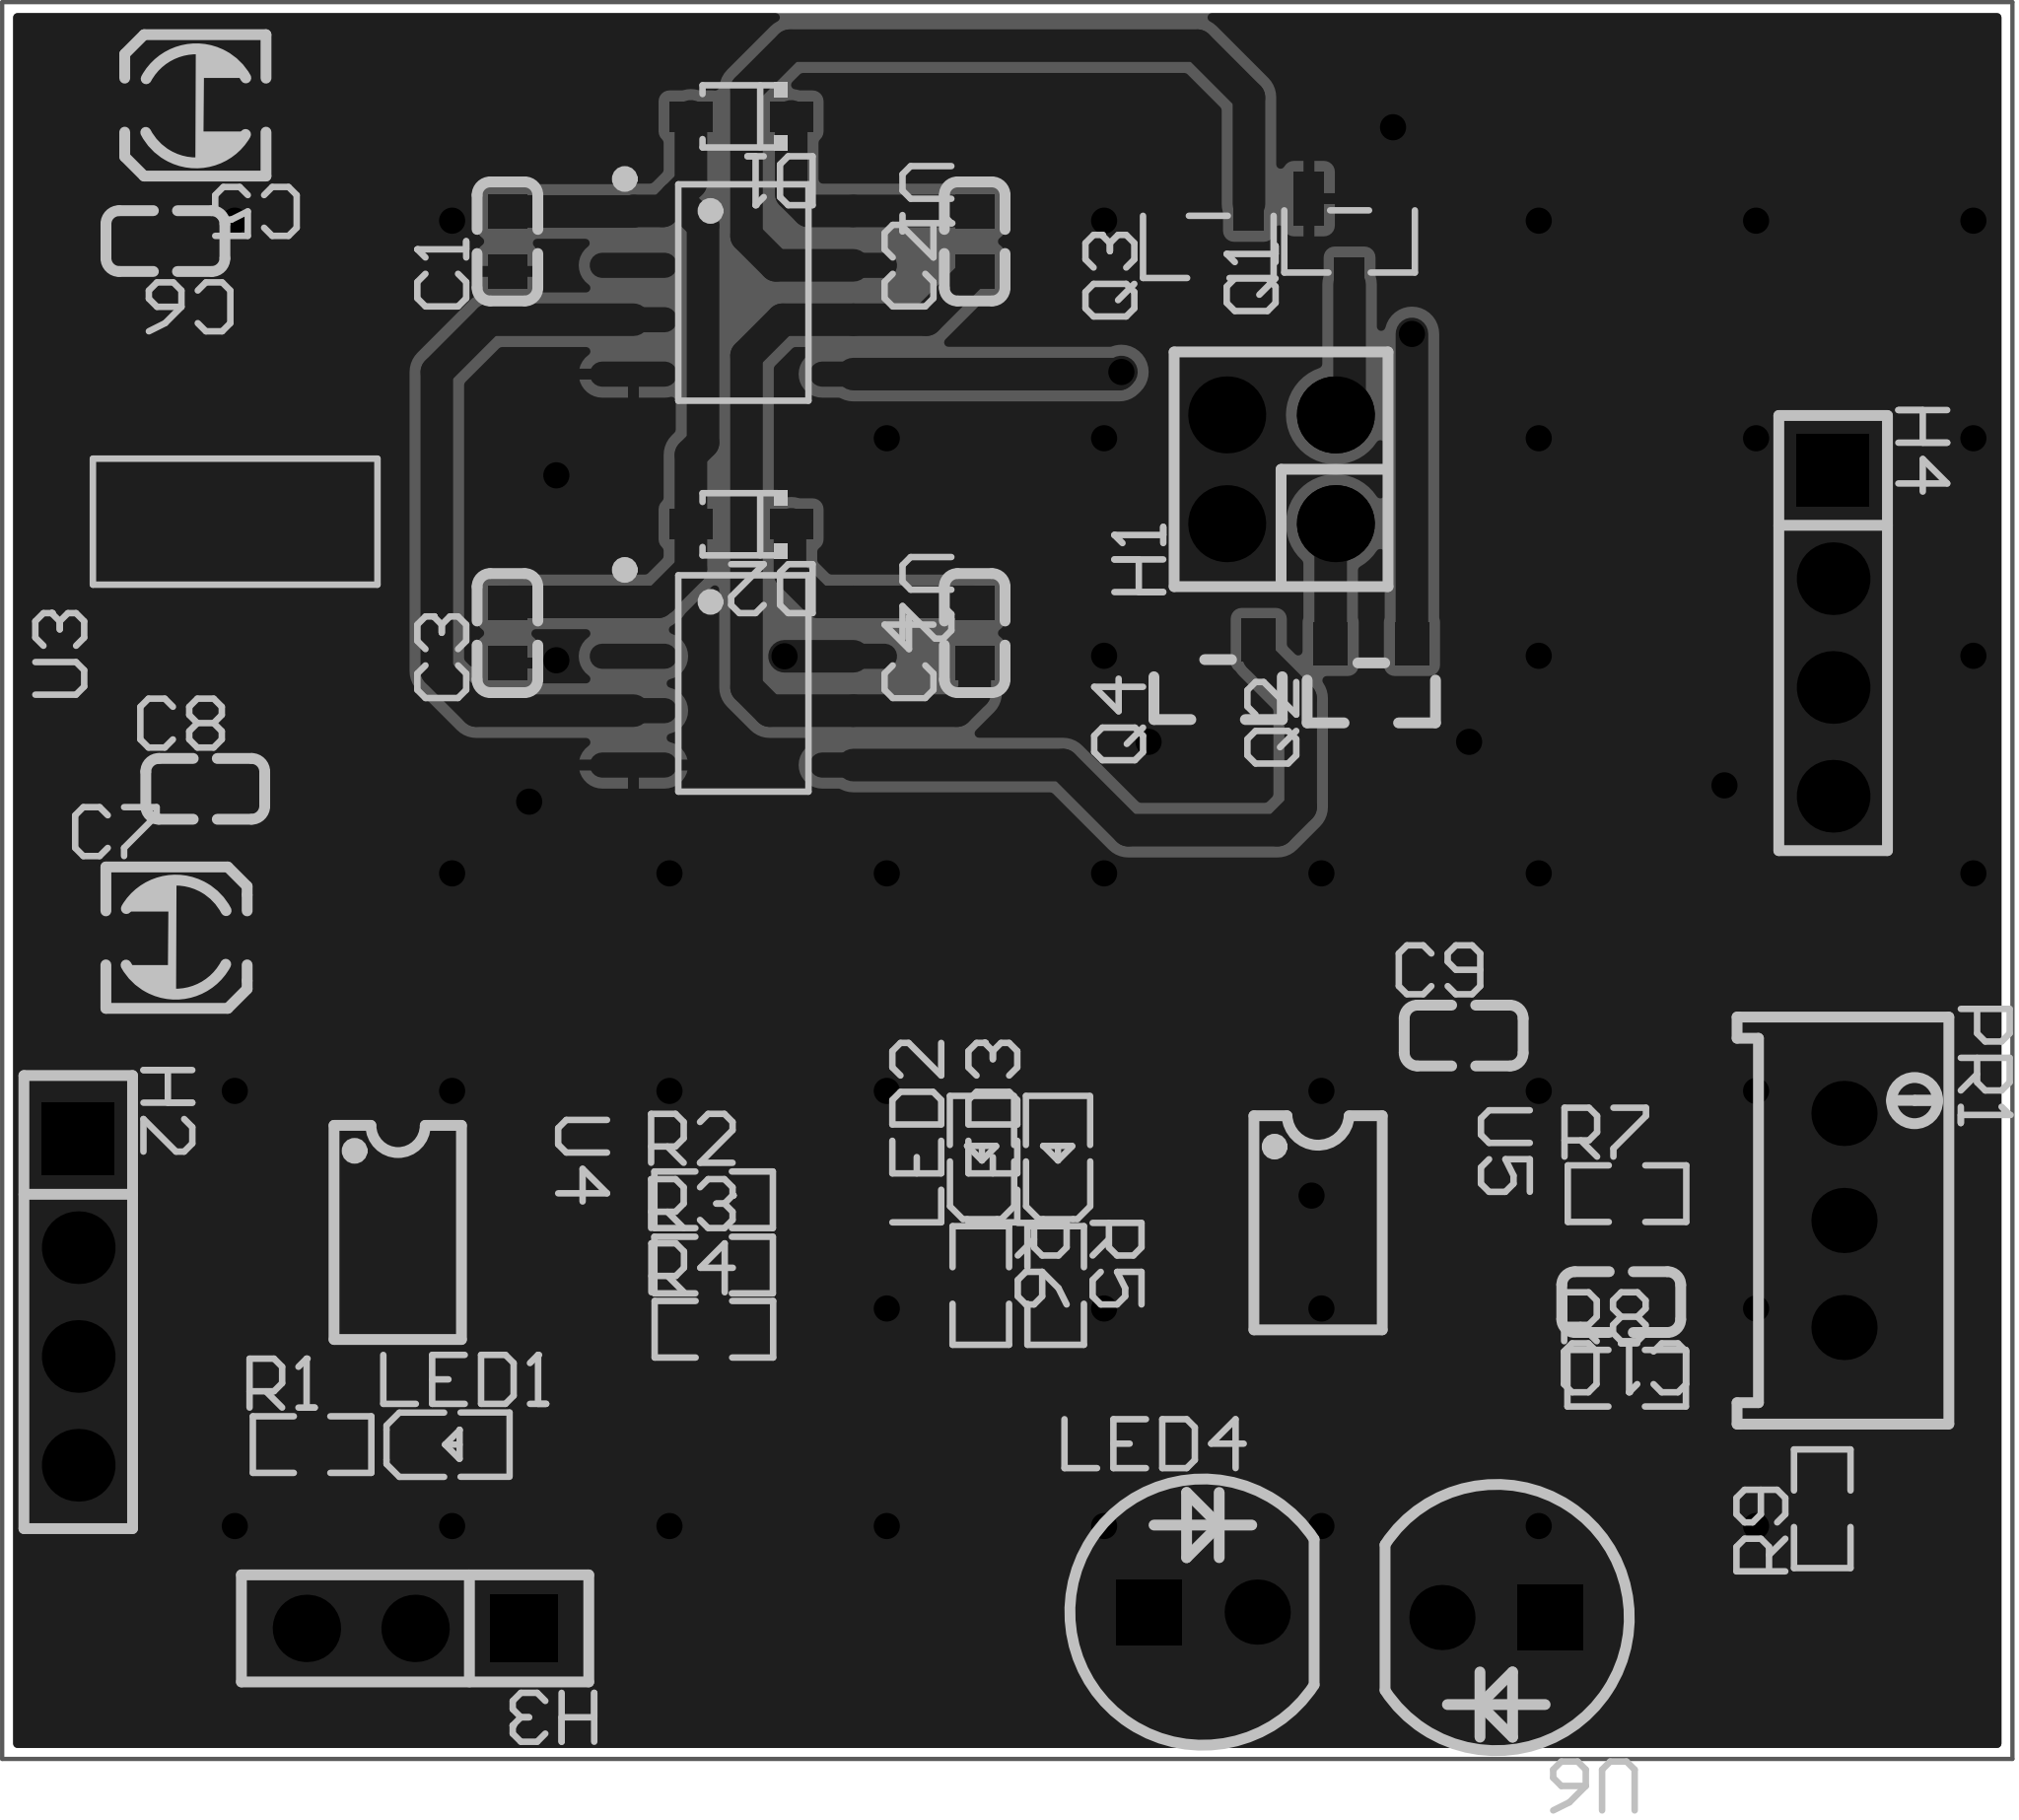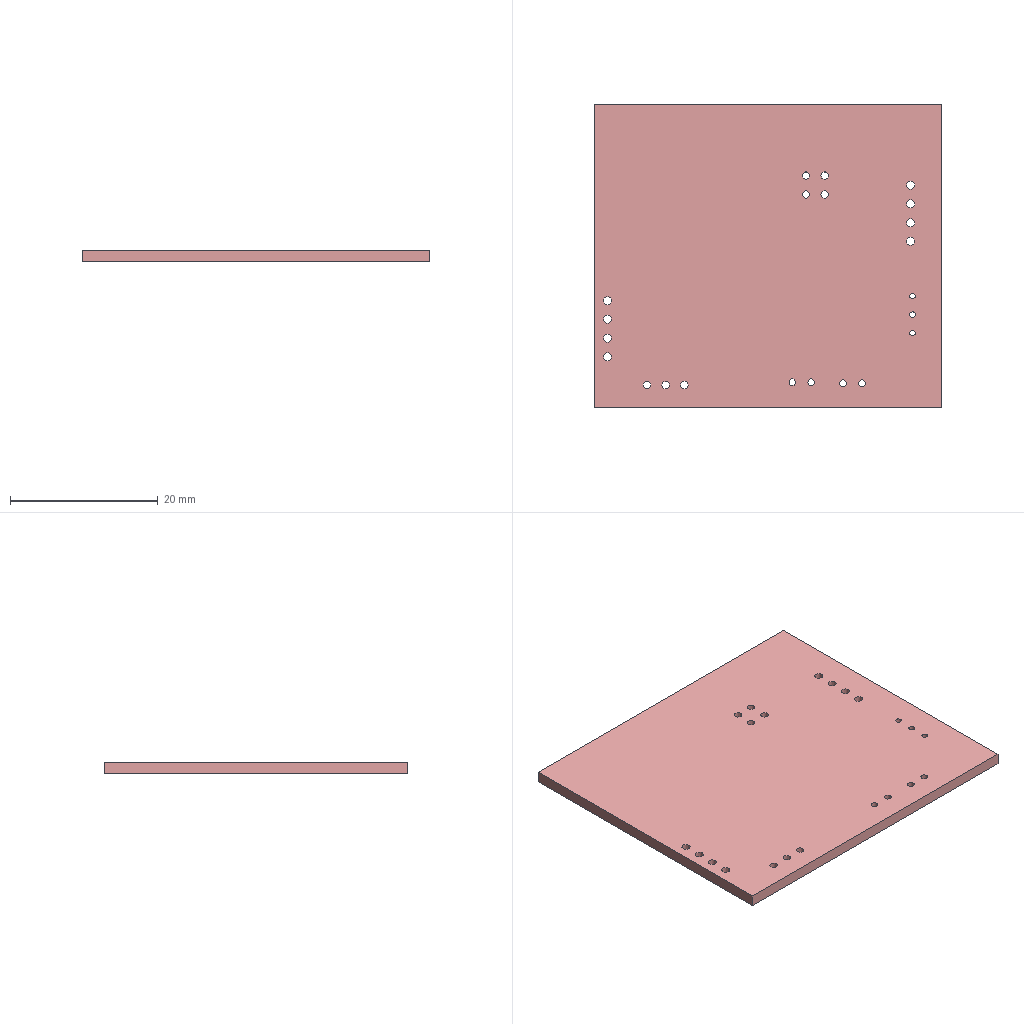Circuit board layout | Altium Designer | box 47 x 41 x 1.6 mm
Layer stack:
# Altium Designer layer stack of  (unit mm; dielectric type: 0 none, 1 core, 2 prepreg, 3 surface material)
index,name,kind,layer,copper_thickness_mm,dielectric_type,dielectric_thickness_mm,dielectric_material,dielectric_constant
0,Top Paste Mask Layer,other,,,,,,
1,Top Silkscreen Layer,other,,,,,,
2,Top Solder Mask Layer,dielectric,,,3,0.01,,3.3
3,Top Layer,copper,Top Layer,0.035,,,,
4,Dielectric1,dielectric,,,3,1.51,FR4,4.5
5,Bottom Layer,copper,Bottom Layer,0.035,,,,
6,Bottom Solder Mask Layer,dielectric,,,3,0.01,,3.3
7,Bottom Silkscreen Layer,other,,,,,,
8,Bottom Paste Mask Layer,other,,,,,,
# drill layer pairs: low layer,high layer
drill_pair,Top Layer,Bottom Layer
Part placement:
Designator,Comment,Layer,Footprint,Center-X(mm),Center-Y(mm),Rotation
C1,100nF,TopLayer,C0603,96.012,118.872,90
C2,100nF,TopLayer,C0603,106.934,118.872,90
C3,100nF,TopLayer,C0603,96.012,109.728,90
C4,100nF,TopLayer,C0603,106.934,109.728,90
C5,10uF,TopLayer,C_Ele_SMD_3x5.4mm,88.717,122.055,180
C6,100nF,TopLayer,C0603,88.017,118.881,180
C7,10uF,TopLayer,C_Ele_SMD_3x5.4mm,88.276,102.611,0
C8,100nF,TopLayer,C0603,88.948,106.09,0
C9,100nF,TopLayer,C0603,118.364,100.33,0
C10,100nF,TopLayer,C0603,122.047,94.107,180
D1,1N5819WS,TopLayer,SOD-323_L1.8-W1.3-LS2.5-RD,101.473,121.793,180
D2,1N5819WS,TopLayer,SOD-323_L1.8-W1.3-LS2.5-RD,101.473,112.268,180
H1,,TopLayer,HDR-TH_4P-P2.54-V-F-R2-C2-S2.54,114.095,113.552,90
H2,,TopLayer,HDR-TH_4P-P2.54-V-F,85.979,94.107,270
H3,,TopLayer,HDR-TH_3P-P2.54-V-F,93.853,86.487,180
H4,,TopLayer,HDR-TH_4P-P2.54-V-M,127,109.728,270
LED1,,TopLayer,LED_0603,94.673,90.772,0
LED2,,TopLayer,LED_0603,107.11,97.532,90
LED3,,TopLayer,LED_0603,108.888,97.532,90
LED4,PT334-6B,TopLayer,LED-TH_BD5.9-P2.54-FD,112.268,86.868,0
PR1,10kΩ,TopLayer,R_3296,127.254,96.012,270
Q1,,TopLayer,SOT-23-3_L2.9-W1.3-P1.90-LS2.4-BR,115.697,118.872,90
Q2,,TopLayer,AO3401A_SOT-23-3,116.205,108.331,90
Q3,,TopLayer,SOT-23-3_L2.9-W1.3-P1.90-LS2.4-BR,112.395,118.745,90
Q4,,TopLayer,AO3401A_SOT-23-3,112.624,108.409,90
R1,1K,TopLayer,R0603,91.445,90.779,0
R2,NC,TopLayer,R0603,100.831,96.495,0
R3,NC,TopLayer,R0603,100.831,94.971,0
R4,NC,TopLayer,R0603,100.838,93.472,0
R5,1K,TopLayer,R0603,108.827,94.494,270
R6,1K,TopLayer,R0603,107.077,94.494,270
R7,10K,TopLayer,R0603,122.183,96.638,0
R8,10K,TopLayer,R0603,122.174,92.329,0
R9,100,TopLayer,R0603,126.746,89.281,90
U1,IR2104STRPBF,TopLayer,SOIC-8_L4.9-W3.9-P1.27-LS6.0-BL,101.527,117.68,270
U2,IR2104STRPBF,TopLayer,SOIC-8_L4.9-W3.9-P1.27-LS6.0-BL,101.527,108.551,270
U3,AMS1117-3.3,TopLayer,SOT-223-3_L6.5-W3.4-P2.30-LS7.0-BR,89.648,112.429,90
U4,1152,TopLayer,SOP-8_L4.9-W3.9-P1.27-LS6.0-BL,93.455,95.733,270
U5,LM393DT,TopLayer,SOIC-8_L5.0-W4.0-P1.27-LS6.0-BL,114.96,95.958,270
U6,DY-IR333C-A,TopLayer,LED-TH_BD5.9-P2.54-FD,119.126,86.741,180
Pad and via stacks:
# Altium Designer via and pad stacks of  (unit mm). Each distinct definition once, with the count of objects using it.
# via: kind,start_layer,end_layer,hole_mm,diameter_mm,mode(0 simple;1 top-mid-bottom;2 full stack),diameter_per_layer,count,example_net
# pad: kind,layer,hole_mm,hole_type(0 round;1 square;2 slot),plating,top_size,top_shape(1 round;2 rect;3 octagon;9 rounded rect),mid_size,bottom_size,mode,footprint,size_per_layer,count,example
pad,Top Layer,0,0,plated,0.8x0.9,2,0.8x0.9,0.8x0.9,0,C0603,,16,C1.2
pad,Top Layer,0,0,plated,1.999x0.8001,2,1.999x0.8001,1.999x0.8001,0,C_Ele_SMD_3x5.4mm,,4,C5.1
pad,Top Layer,0,0,plated,1x0.7,2,1x0.7,1x0.7,0,SOD-323_L1.8-W1.3-LS2.5-RD,,4,D1.1
pad,Top Layer,0,0,plated,0.8001x0.8001,2,0.8001x0.8001,0.8001x0.8001,0,LED_0603,,6,LED1.1
pad,Top Layer,0,0,plated,1.25x0.7,2,1.25x0.7,1.25x0.7,0,SOT-23-3_L2.9-W1.3-P1.90-LS2.4-BR,,6,Q1.1
pad,Top Layer,0,0,plated,1x0.8,2,1x0.8,1x0.8,0,AO3401A_SOT-23-3,,6,Q2.2
pad,Top Layer,0,0,plated,0.8065x0.864,2,0.8065x0.864,0.8065x0.864,0,R0603,,18,R1.2
pad,Top Layer,0,0,plated,0.588x2.045,1,0.588x2.045,0.588x2.045,0,SOIC-8_L4.9-W3.9-P1.27-LS6.0-BL,,16,U1.5
pad,Top Layer,0,0,plated,2.5x1.1,2,2.5x1.1,2.5x1.1,0,SOT-223-3_L6.5-W3.4-P2.30-LS7.0-BR,,3,U3.1
pad,Top Layer,0,0,plated,2.34x3.6,2,2.34x3.6,2.34x3.6,0,SOT-223-3_L6.5-W3.4-P2.30-LS7.0-BR,,1,U3.4
pad,Top Layer,0,0,plated,0.63x1.865,1,0.63x1.865,0.63x1.865,0,SOP-8_L4.9-W3.9-P1.27-LS6.0-BL,,8,U4.1
pad,Top Layer,0,0,plated,0.5684x1.95,1,0.5684x1.95,0.5684x1.95,0,SOIC-8_L5.0-W4.0-P1.27-LS6.0-BL,,8,U5.1
pad,Multi-Layer,1,0,plated,1.8x1.8,1,1.8x1.8,1.8x1.8,0,HDR-TH_4P-P2.54-V-F-R2-C2-S2.54,,4,H1.4
pad,Multi-Layer,1.1,0,plated,1.7x1.7,2,1.7x1.7,1.7x1.7,0,HDR-TH_4P-P2.54-V-F,,1,H2.1
pad,Multi-Layer,1.1,0,plated,1.7x1.7,1,1.7x1.7,1.7x1.7,0,HDR-TH_4P-P2.54-V-F,,3,H2.2
pad,Multi-Layer,1.02,0,plated,1.575x1.575,1,1.575x1.575,1.575x1.575,0,HDR-TH_3P-P2.54-V-F,,2,H3.3
pad,Multi-Layer,1.02,0,plated,1.575x1.575,2,1.575x1.575,1.575x1.575,0,HDR-TH_3P-P2.54-V-F,,1,H3.1
pad,Multi-Layer,1.1,0,plated,1.7x1.7,2,1.7x1.7,1.7x1.7,0,HDR-TH_4P-P2.54-V-M,,1,H4.1
pad,Multi-Layer,1.1,0,plated,1.7x1.7,1,1.7x1.7,1.7x1.7,0,HDR-TH_4P-P2.54-V-M,,3,H4.2
pad,Multi-Layer,0.9144,0,plated,1.524x1.524,1,1.524x1.524,1.524x1.524,0,LED-TH_BD5.9-P2.54-FD,,2,LED4.2
pad,Multi-Layer,0.9144,0,plated,1.524x1.524,2,1.524x1.524,1.524x1.524,0,LED-TH_BD5.9-P2.54-FD,,2,LED4.1
pad,Multi-Layer,0.762,0,plated,1.524x1.524,1,1.524x1.524,1.524x1.524,0,R_3296,,3,PR1.2
via,Top Layer,Bottom Layer,0.3048,0.61,0,,51,MOS1-H
Copper pours:
name,layer,net,type(0 solid;1 hatched;2 none)
Top Layer-GND,Top Layer,GND,0
Bottom Layer-GND,Bottom Layer,GND,0